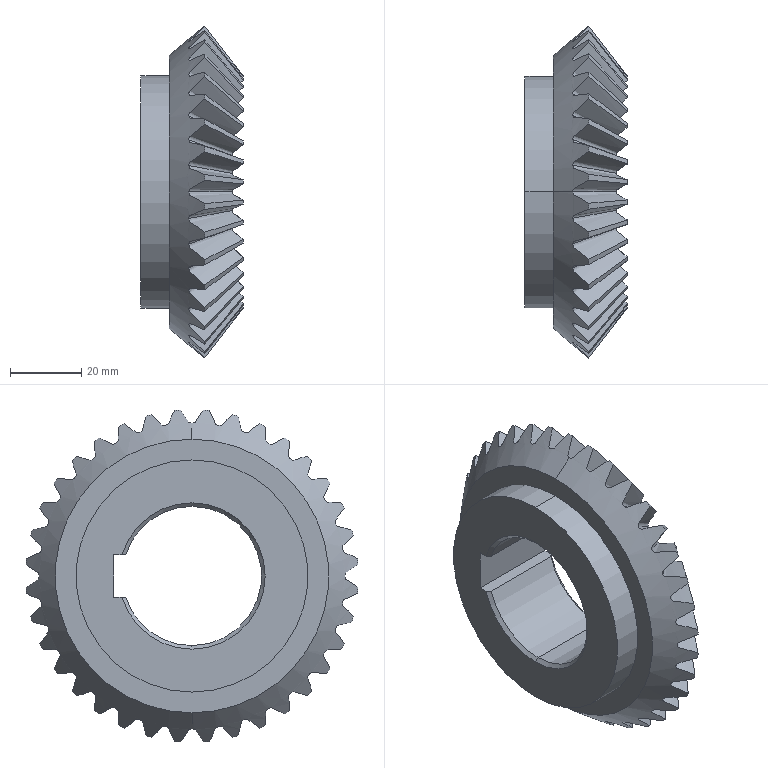Part | SolidWorks | features ICE 2, BlendCut 1, Chamfer 1, CirPattern 1, RefAxis 1, Revolution 1 | 1 solid | 164 faces | box 28.614 x 92.976 x 92.976 mm | volume 84725 mm3 | cone 80 | spline 72 | plane 7 | cylinder 5 | commonest cylinder face diameters 39 x3 65 x2